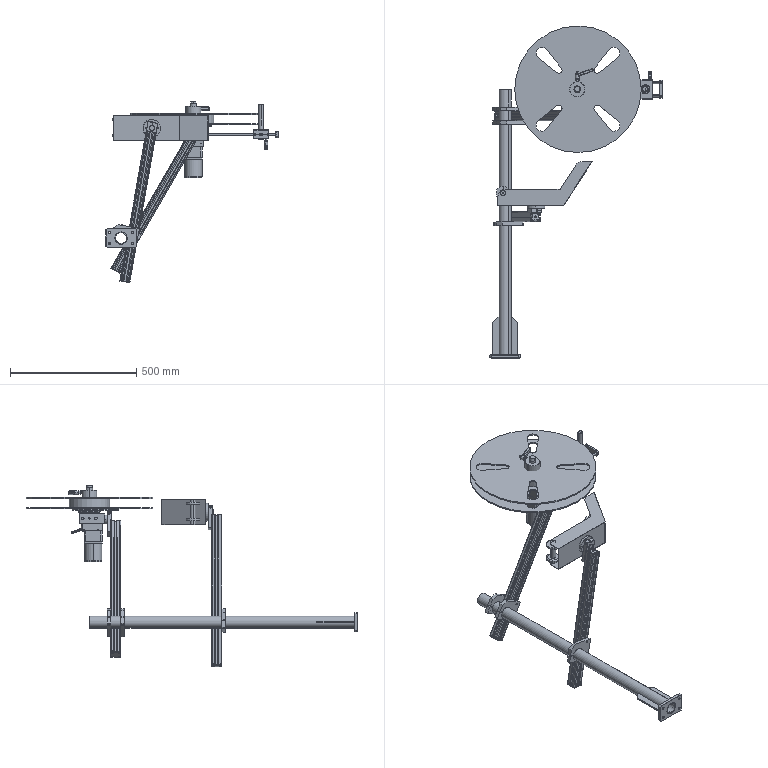Part | NX | 43 solids | 1494 faces | box 680.718 x 1312 x 717.346 mm | volume 6126182 mm3 | cylinder 582 | plane 522 | cone 293 | torus 57 | spline 30 | sphere 10 | commonest cylinder face diameters 4.2 x44 10 x39 8 x36 6.5 x28 25 x28 19 x26